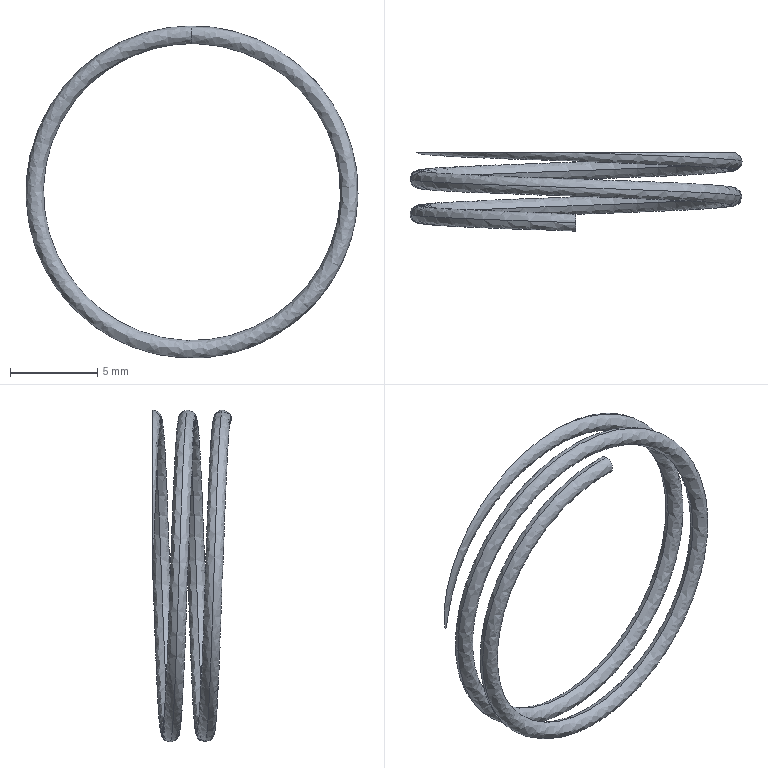Part | STEP file | 0217_002_WR18-20 | 1 solid | 4 faces | box 19 x 4.5 x 19 mm | volume 92.511 mm3 | spline 2 | plane 2